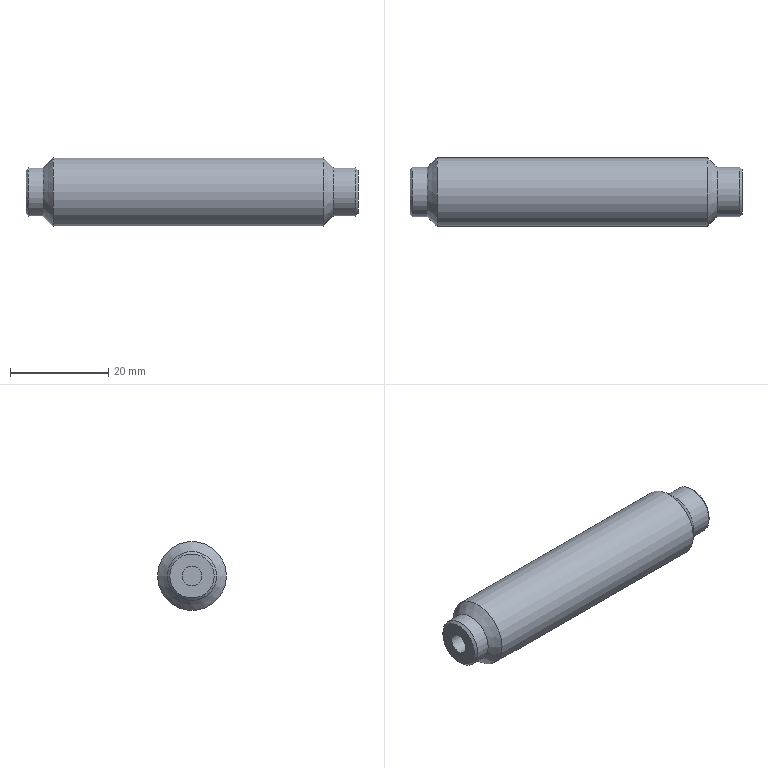Part | NX | features BODY_5003_019_C-AC1412S 2 | 1 solid | 11 faces | box 67.5 x 14 x 14 mm | volume 9382 mm3 | cone 4 | cylinder 4 | plane 3 | commonest cylinder face diameters 10 x2 4 x1 14 x1
STEP:
#1=CARTESIAN_POINT('',(41.1,-141.5,-223.));
#2=VERTEX_POINT('',#1);
#3=CARTESIAN_POINT('',(41.1,-137.,-223.));
#4=DIRECTION('',(-1.,0.,0.));
#5=DIRECTION('',(0.,-1.,0.));
#6=AXIS2_PLACEMENT_3D('',#3,#4,#5);
#7=CIRCLE('',#6,4.5);
#8=EDGE_CURVE('',#2,#2,#7,.T.);
#9=ORIENTED_EDGE('',*,*,#8,.T.);
#10=EDGE_LOOP('',(#9));
#11=FACE_BOUND('',#10,.T.);
#12=CARTESIAN_POINT('',(41.1,-139.,-223.));
#13=VERTEX_POINT('',#12);
#14=CARTESIAN_POINT('',(41.1,-137.,-223.));
#15=DIRECTION('',(-1.,0.,0.));
#16=DIRECTION('',(0.,-1.,0.));
#17=AXIS2_PLACEMENT_3D('',#14,#15,#16);
#18=CIRCLE('',#17,2.);
#19=EDGE_CURVE('',#13,#13,#18,.T.);
#20=ORIENTED_EDGE('',*,*,#19,.F.);
#21=EDGE_LOOP('',(#20));
#22=FACE_BOUND('',#21,.T.);
#23=CARTESIAN_POINT('',(41.1,-137.,-223.));
#24=DIRECTION('',(-1.,0.,0.));
#25=DIRECTION('',(0.,-1.,0.));
#26=AXIS2_PLACEMENT_3D('',#23,#24,#25);
#27=PLANE('',#26);
#28=ADVANCED_FACE('',(#11,#22),#27,.T.);
#29=CARTESIAN_POINT('',(46.6,-144.,-223.));
#30=VERTEX_POINT('',#29);
#31=CARTESIAN_POINT('',(46.6,-137.,-223.));
#32=DIRECTION('',(-1.,0.,0.));
#33=DIRECTION('',(0.,-1.,0.));
#34=AXIS2_PLACEMENT_3D('',#31,#32,#33);
#35=CIRCLE('',#34,7.);
#36=EDGE_CURVE('',#30,#30,#35,.T.);
#37=ORIENTED_EDGE('',*,*,#36,.T.);
#38=EDGE_LOOP('',(#37));
#39=FACE_BOUND('',#38,.T.);
#40=CARTESIAN_POINT('',(44.6,-142.,-223.));
#41=VERTEX_POINT('',#40);
#42=CARTESIAN_POINT('',(44.6,-137.,-223.));
#43=DIRECTION('',(-1.,0.,0.));
#44=DIRECTION('',(0.,-1.,0.));
#45=AXIS2_PLACEMENT_3D('',#42,#43,#44);
#46=CIRCLE('',#45,5.);
#47=EDGE_CURVE('',#41,#41,#46,.T.);
#48=ORIENTED_EDGE('',*,*,#47,.F.);
#49=EDGE_LOOP('',(#48));
#50=FACE_BOUND('',#49,.T.);
#51=CARTESIAN_POINT('',(44.6,-137.,-223.));
#52=DIRECTION('',(1.,0.,0.));
#53=DIRECTION('',(0.,1.,0.));
#54=AXIS2_PLACEMENT_3D('',#51,#52,#53);
#55=CONICAL_SURFACE('',#54,5.,0.7854);
#56=ADVANCED_FACE('',(#39,#50),#55,.T.);
#57=CARTESIAN_POINT('',(101.6,-144.,-223.));
#58=VERTEX_POINT('',#57);
#59=CARTESIAN_POINT('',(101.6,-137.,-223.));
#60=DIRECTION('',(-1.,0.,0.));
#61=DIRECTION('',(0.,-1.,0.));
#62=AXIS2_PLACEMENT_3D('',#59,#60,#61);
#63=CIRCLE('',#62,7.);
#64=EDGE_CURVE('',#58,#58,#63,.T.);
#65=ORIENTED_EDGE('',*,*,#64,.T.);
#66=EDGE_LOOP('',(#65));
#67=FACE_BOUND('',#66,.T.);
#68=ORIENTED_EDGE('',*,*,#36,.F.);
#69=EDGE_LOOP('',(#68));
#70=FACE_BOUND('',#69,.T.);
#71=CARTESIAN_POINT('',(37.725,-137.,-223.));
#72=DIRECTION('',(-1.,0.,0.));
#73=DIRECTION('',(0.,-1.,0.));
#74=AXIS2_PLACEMENT_3D('',#71,#72,#73);
#75=CYLINDRICAL_SURFACE('',#74,7.);
#76=ADVANCED_FACE('',(#67,#70),#75,.T.);
#77=CARTESIAN_POINT('',(103.6,-142.,-223.));
#78=VERTEX_POINT('',#77);
#79=CARTESIAN_POINT('',(103.6,-137.,-223.));
#80=DIRECTION('',(-1.,0.,0.));
#81=DIRECTION('',(0.,-1.,0.));
#82=AXIS2_PLACEMENT_3D('',#79,#80,#81);
#83=CIRCLE('',#82,5.);
#84=EDGE_CURVE('',#78,#78,#83,.T.);
#85=ORIENTED_EDGE('',*,*,#84,.T.);
#86=EDGE_LOOP('',(#85));
#87=FACE_BOUND('',#86,.T.);
#88=ORIENTED_EDGE('',*,*,#64,.F.);
#89=EDGE_LOOP('',(#88));
#90=FACE_BOUND('',#89,.T.);
#91=CARTESIAN_POINT('',(101.6,-137.,-223.));
#92=DIRECTION('',(-1.,0.,0.));
#93=DIRECTION('',(0.,-1.,0.));
#94=AXIS2_PLACEMENT_3D('',#91,#92,#93);
#95=CONICAL_SURFACE('',#94,7.,0.7854);
#96=ADVANCED_FACE('',(#87,#90),#95,.T.);
#97=CARTESIAN_POINT('',(108.1,-142.,-223.));
#98=VERTEX_POINT('',#97);
#99=CARTESIAN_POINT('',(108.1,-137.,-223.));
#100=DIRECTION('',(-1.,0.,0.));
#101=DIRECTION('',(0.,-1.,0.));
#102=AXIS2_PLACEMENT_3D('',#99,#100,#101);
#103=CIRCLE('',#102,5.);
#104=EDGE_CURVE('',#98,#98,#103,.T.);
#105=ORIENTED_EDGE('',*,*,#104,.T.);
#106=EDGE_LOOP('',(#105));
#107=FACE_BOUND('',#106,.T.);
#108=ORIENTED_EDGE('',*,*,#84,.F.);
#109=EDGE_LOOP('',(#108));
#110=FACE_BOUND('',#109,.T.);
#111=CARTESIAN_POINT('',(37.725,-137.,-223.));
#112=DIRECTION('',(-1.,0.,0.));
#113=DIRECTION('',(0.,-1.,0.));
#114=AXIS2_PLACEMENT_3D('',#111,#112,#113);
#115=CYLINDRICAL_SURFACE('',#114,5.);
#116=ADVANCED_FACE('',(#107,#110),#115,.T.);
#117=ORIENTED_EDGE('',*,*,#104,.F.);
#118=EDGE_LOOP('',(#117));
#119=FACE_BOUND('',#118,.T.);
#120=CARTESIAN_POINT('',(108.6,-141.5,-223.));
#121=VERTEX_POINT('',#120);
#122=CARTESIAN_POINT('',(108.6,-137.,-223.));
#123=DIRECTION('',(-1.,0.,0.));
#124=DIRECTION('',(0.,-1.,0.));
#125=AXIS2_PLACEMENT_3D('',#122,#123,#124);
#126=CIRCLE('',#125,4.5);
#127=EDGE_CURVE('',#121,#121,#126,.T.);
#128=ORIENTED_EDGE('',*,*,#127,.T.);
#129=EDGE_LOOP('',(#128));
#130=FACE_BOUND('',#129,.T.);
#131=CARTESIAN_POINT('',(108.6,-137.,-223.));
#132=DIRECTION('',(-1.,0.,0.));
#133=DIRECTION('',(0.,-1.,0.));
#134=AXIS2_PLACEMENT_3D('',#131,#132,#133);
#135=CONICAL_SURFACE('',#134,4.5,0.7854);
#136=ADVANCED_FACE('',(#119,#130),#135,.T.);
#137=ORIENTED_EDGE('',*,*,#127,.F.);
#138=EDGE_LOOP('',(#137));
#139=FACE_BOUND('',#138,.T.);
#140=CARTESIAN_POINT('',(108.6,-137.,-218.5));
#141=DIRECTION('',(1.,0.,0.));
#142=DIRECTION('',(0.,1.,0.));
#143=AXIS2_PLACEMENT_3D('',#140,#141,#142);
#144=PLANE('',#143);
#145=ADVANCED_FACE('',(#139),#144,.T.);
#146=CARTESIAN_POINT('',(41.6,-142.,-223.));
#147=VERTEX_POINT('',#146);
#148=CARTESIAN_POINT('',(41.6,-137.,-223.));
#149=DIRECTION('',(-1.,0.,0.));
#150=DIRECTION('',(0.,-1.,0.));
#151=AXIS2_PLACEMENT_3D('',#148,#149,#150);
#152=CIRCLE('',#151,5.);
#153=EDGE_CURVE('',#147,#147,#152,.T.);
#154=ORIENTED_EDGE('',*,*,#153,.T.);
#155=EDGE_LOOP('',(#154));
#156=FACE_BOUND('',#155,.T.);
#157=ORIENTED_EDGE('',*,*,#8,.F.);
#158=EDGE_LOOP('',(#157));
#159=FACE_BOUND('',#158,.T.);
#160=CARTESIAN_POINT('',(41.1,-137.,-223.));
#161=DIRECTION('',(1.,0.,0.));
#162=DIRECTION('',(0.,1.,0.));
#163=AXIS2_PLACEMENT_3D('',#160,#161,#162);
#164=CONICAL_SURFACE('',#163,4.5,0.7854);
#165=ADVANCED_FACE('',(#156,#159),#164,.T.);
#166=ORIENTED_EDGE('',*,*,#47,.T.);
#167=EDGE_LOOP('',(#166));
#168=FACE_BOUND('',#167,.T.);
#169=ORIENTED_EDGE('',*,*,#153,.F.);
#170=EDGE_LOOP('',(#169));
#171=FACE_BOUND('',#170,.T.);
#172=CARTESIAN_POINT('',(37.725,-137.,-223.));
#173=DIRECTION('',(-1.,0.,0.));
#174=DIRECTION('',(0.,-1.,0.));
#175=AXIS2_PLACEMENT_3D('',#172,#173,#174);
#176=CYLINDRICAL_SURFACE('',#175,5.);
#177=ADVANCED_FACE('',(#168,#171),#176,.T.);
#178=CARTESIAN_POINT('',(57.1,-139.,-223.));
#179=VERTEX_POINT('',#178);
#180=CARTESIAN_POINT('',(57.1,-137.,-223.));
#181=DIRECTION('',(-1.,0.,0.));
#182=DIRECTION('',(0.,-1.,0.));
#183=AXIS2_PLACEMENT_3D('',#180,#181,#182);
#184=CIRCLE('',#183,2.);
#185=EDGE_CURVE('',#179,#179,#184,.T.);
#186=ORIENTED_EDGE('',*,*,#185,.T.);
#187=EDGE_LOOP('',(#186));
#188=FACE_BOUND('',#187,.T.);
#189=CARTESIAN_POINT('',(57.1,-137.,-223.));
#190=DIRECTION('',(-1.,0.,0.));
#191=DIRECTION('',(0.,-1.,0.));
#192=AXIS2_PLACEMENT_3D('',#189,#190,#191);
#193=PLANE('',#192);
#194=ADVANCED_FACE('',(#188),#193,.T.);
#195=ORIENTED_EDGE('',*,*,#19,.T.);
#196=EDGE_LOOP('',(#195));
#197=FACE_BOUND('',#196,.T.);
#198=ORIENTED_EDGE('',*,*,#185,.F.);
#199=EDGE_LOOP('',(#198));
#200=FACE_BOUND('',#199,.T.);
#201=CARTESIAN_POINT('',(37.725,-137.,-223.));
#202=DIRECTION('',(-1.,0.,0.));
#203=DIRECTION('',(0.,-1.,0.));
#204=AXIS2_PLACEMENT_3D('',#201,#202,#203);
#205=CYLINDRICAL_SURFACE('',#204,2.);
#206=ADVANCED_FACE('',(#197,#200),#205,.F.);
#207=CLOSED_SHELL('',(#28,#56,#76,#96,#116,#136,#145,#165,#177,#194,#206));
#208=MANIFOLD_SOLID_BREP('',#207);
#209=(LENGTH_UNIT()NAMED_UNIT(*)SI_UNIT(.MILLI.,.METRE.));
#210=UNCERTAINTY_MEASURE_WITH_UNIT(LENGTH_MEASURE(0.00001),#209,'','');
#211=(NAMED_UNIT(*)PLANE_ANGLE_UNIT()SI_UNIT($,.RADIAN.));
#212=(NAMED_UNIT(*)SI_UNIT($,.STERADIAN.)SOLID_ANGLE_UNIT());
#213=(GEOMETRIC_REPRESENTATION_CONTEXT(3)GLOBAL_UNCERTAINTY_ASSIGNED_CONTEXT((#210))GLOBAL_UNIT_ASSIGNED_CONTEXT((#209,#211,#212))REPRESENTATION_CONTEXT('',''));
#214=ADVANCED_BREP_SHAPE_REPRESENTATION('',(#208),#213);